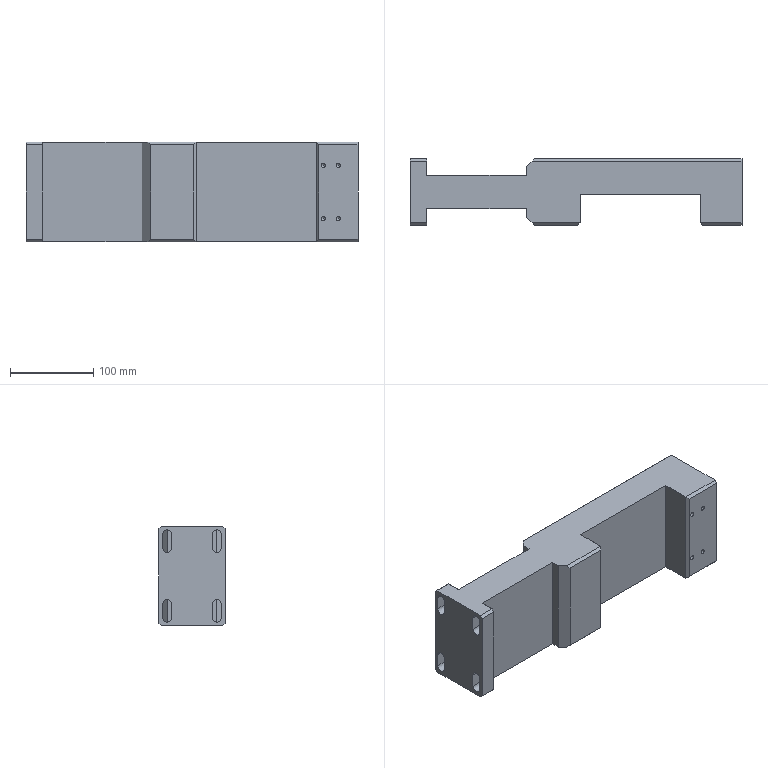CAM job | NX | 3+2 milling, drilling | part box 400 x 80 x 120 mm | stock box 405 x 85 x 125 mm
Tools:
number,name,description,diameter,corner_radius,flute_length,length,flutes
9,D10,平底铣刀-粗,10.0,0.0,35.0,75.0,2
17,D16,平底铣刀-粗,16.0,0.0,50.0,75.0,2
10,D10-J,平底铣刀-精,10.0,0.0,35.0,75.0,2
18,D16-J,平底铣刀-精,16.0,0.0,50.0,75.0,2
19,D6R0.5,圆鼻刀-粗,6.0,0.5,50.0,75.0,2
1,D80R0.8_FLYCUTTER,圆鼻刀-粗,80.0,0.8,50.0,75.0,2
1,D80R0.8_FLYCUTTER-J,圆鼻刀-精,80.0,0.8,50.0,75.0,2
2,D6_CHAMFERTOOL,倒角刀,6.0,0.0,3.0,25.0,2
24,D10_CHAMFERTOOL,倒角刀,10.0,0.0,5.0,75.0,2
23,M6X1.0,丝锥,5.0,0.0,35.0,50.0,2
15,ZT5,钻头,5.0,0.0,35.0,50.0,2
Operations:
program,operation,operation_type,tool,method,geometry_group,spindle_rpm,surface_speed,feed_per_tooth,feed_cut,feed_plunge,cut_length_mm,path_length_mm,cut_time_min,machine_time_min
B,FLOORWALL_FLYFACEROUGH_COPY,VolumeBased25DMillingOperation,D80R0.8_FLYCUTTER,LAYERROUGH-DEPTHK-STEPG,W-B,5000.0,1256.637,0.3,3000.0,100.0,9417.186,9967.757,3.139,3.194
B,FLOORWALL_FLYFACEFINISH_COPY,VolumeBased25DMillingOperation,D80R0.8_FLYCUTTER-J,SIDEFINISH-DEPTHK-STEPG,W-B,5000.0,1256.637,0.1,1000.0,100.0,1045.766,1081.766,1.046,1.049
B,CAVITY_ROUGH-MID_COPY_COPY,CavityMilling,D10,LAYERROUGH-DEPTHK-STEPG,W-B,8000.0,251.327,0.375,6000.0,100.0,183531.242,190654.782,30.588,31.591
B,ZLEVEL_FINISH_ZIGZAGSTEEP_COPY_COPY,ZLevelMilling,D6R0.5,ZLEVELSTEEP-DEPTHK-STEPG,W-B,7000.0,131.947,0.3571,5000.0,100.0,15070.33,15110.015,3.014,3.018
B,CENTERDRILL-DEPTH0.8_2,Operation,D6_CHAMFERTOOL,NONE,W-B,8000.0,150.796,0.0312,500.0,90.0,7.2,157.463,0.0144,0.0294
B,BLINDCONE-M6_TAPDRILL_2,Operation,ZT5,NONE,W-B,2500.0,39.27,0.06,300.0,90.0,78.009,299.08,0.26,0.2821
B,MILLCHAMFER_2,PlanarMilling,D6_CHAMFERTOOL,METHOD,W-B,8000.0,150.796,0.0375,600.0,100.0,75.821,342.245,0.1264,0.153
B,PLANEDEBURR6X45L_COPY,SurfaceContour,D10_CHAMFERTOOL,STEEPCHAMFER-DEPTH0-STEPG,W-B,6500.0,122.519,0.1154,1500.0,100.0,1074.568,2514.709,0.7164,0.8604
B,FLOORWALL_CHAMFER_COPY_COPY,VolumeBased25DMillingOperation,D10_CHAMFERTOOL,STEEPCHAMFER-DEPTH0-STEPG,W-B,6500.0,122.519,0.1154,1500.0,100.0,569.848,1329.606,0.3799,0.4559
B,BLINDCONE-TAP_M6_2,Operation,M6X1.0,METHOD,W-B,500.0,7.854,0.001,1.0,90.0,64.0,271.063,64.0,64.021
B,FLOORWALL_FINISH_BOTTOM-MID_COPY_1,VolumeBased25DMillingOperation,D10-J,FINISHSTEPDEPTHOFF,W-B,8000.0,251.32,0.0625,1000.0,100.0,3090.54,3157.14,3.091,3.097
B,FLOORWALL_FINISH_BOTTOM-MID_COPY_2,VolumeBased25DMillingOperation,D10-J,FINISHSTEPDEPTHOFF,W-B,7000.0,175.0,0.0536,1500.0,100.0,3761.463,3862.063,2.508,2.518
B,FLOORWALL_FINISH_SIDE-MID-SELBOTTOM_COPY_1,VolumeBased25DMillingOperation,D10-J,SIDEFINISH-DEPTHK-STEPG,W-B,8000.0,251.32,0.0625,1000.0,100.0,278.48,463.017,0.2785,0.2969
B,FLOORWALL_FINISH_SIDE-MID-SELBOTTOM_COPY_2,VolumeBased25DMillingOperation,D10-J,SIDEFINISH-DEPTHK-STEPG,W-B,8000.0,251.32,0.0625,1000.0,100.0,556.959,1141.416,0.557,0.6154
A,TOPFACE,FaceMilling,D80R0.8_FLYCUTTER,SIDEFINISH-DEPTHK-STEPG,W-A,5000.0,1256.637,0.1,1000.0,100.0,1040.667,1076.667,1.041,1.044
A,CONTOUR_ROUGH_2,VolumeBased25DMillingOperation,D16,METHOD,W-A,5000.0,251.327,0.5,5000.0,80.0,89454.829,89573.829,17.891,17.903
A,CAVITY_ROUGH-MID_COPY,CavityMilling,D10,LAYERROUGH-DEPTHK-STEPG,W-A,8000.0,251.327,0.375,6000.0,100.0,95824.813,99285.81,15.971,16.483
A,CENTERDRILL-DEPTH0.8,Operation,D6_CHAMFERTOOL,NONE,W-A,8000.0,150.796,0.0312,500.0,90.0,7.2,157.463,0.0144,0.0294
A,BLINDCONE-M6_TAPDRILL,Operation,ZT5,NONE,W-A,2500.0,39.27,0.06,300.0,90.0,78.009,299.08,0.26,0.2821
A,ZLEVEL_FINISH_ZIGZAGSTEEP_COPY,ZLevelMilling,D6R0.5,ZLEVELSTEEP-DEPTHK-STEPG,W-A,7000.0,131.947,0.3571,5000.0,100.0,14948.542,14980.103,2.99,2.993
A,BODYONLY,SurfaceContour,D6_CHAMFERTOOL,METHOD,W-A,8000.0,150.796,0.1875,3000.0,100.0,673.71,1684.081,0.2246,0.3256
A,MILLCHAMFER_1,PlanarMilling,D6_CHAMFERTOOL,METHOD,W-A,8000.0,150.796,0.0375,600.0,100.0,75.821,342.245,0.1264,0.153
A,FLOORWALL_CHAMFER_COPY,VolumeBased25DMillingOperation,D10_CHAMFERTOOL,STEEPCHAMFER-DEPTH0-STEPG,W-A,6500.0,122.519,0.1154,1500.0,100.0,614.248,1148.646,0.4095,0.4629
A,BLINDCONE-TAP_M6,Operation,M6X1.0,METHOD,W-A,500.0,7.854,0.001,1.0,90.0,64.0,271.063,64.0,64.021
A,FLOORWALL_FINISH_BOTTOM-MID_COPY,VolumeBased25DMillingOperation,D10-J,FINISHSTEPDEPTHOFF,W-A,8000.0,251.32,0.0625,1000.0,100.0,3090.54,3148.34,3.091,3.096
A,FLOORWALL_FINISH_SIDE-MID-SELBOTTOM_COPY,VolumeBased25DMillingOperation,D10-J,SIDEFINISH-DEPTHK-STEPG,W-A,8000.0,251.32,0.0625,1000.0,100.0,278.48,453.817,0.2785,0.296
A,CONTOUR_SEMI_2,VolumeBased25DMillingOperation,D16-J,METHOD,W-A,5000.0,251.327,0.1,1000.0,100.0,5476.257,6164.298,5.476,5.545